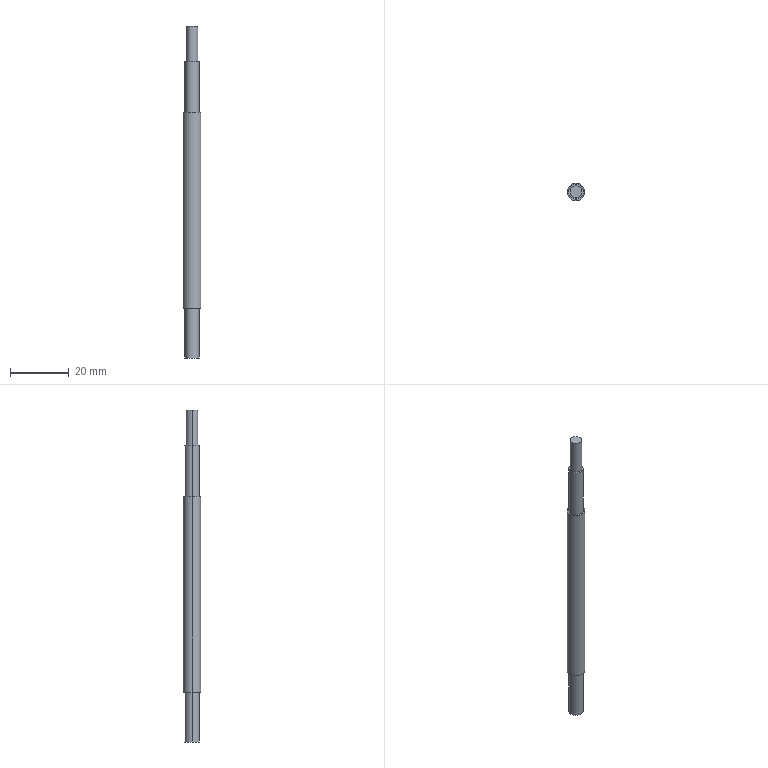Part | SolidWorks | features ICE 3, Extrusion 1 | 1 solid | 13 faces | box 6 x 6 x 113.5 mm | volume 2723 mm3 | cylinder 8 | plane 5 | commonest cylinder face diameters 5 x4 4 x2 6 x2
STEP:
#1=CARTESIAN_POINT('',(2.,0.,113.5));
#2=VERTEX_POINT('',#1);
#3=CARTESIAN_POINT('',(-2.,0.,113.5));
#4=VERTEX_POINT('',#3);
#5=CARTESIAN_POINT('',(0.,0.,113.5));
#6=DIRECTION('',(0.,0.,1.));
#7=DIRECTION('',(1.,0.,0.));
#8=AXIS2_PLACEMENT_3D('',#5,#6,#7);
#9=CIRCLE('',#8,2.);
#10=EDGE_CURVE('',#2,#4,#9,.T.);
#11=ORIENTED_EDGE('',*,*,#10,.F.);
#12=CARTESIAN_POINT('',(2.,0.,101.5));
#13=VERTEX_POINT('',#12);
#14=CARTESIAN_POINT('',(2.,0.,113.5));
#15=DIRECTION('',(0.,0.,-1.));
#16=VECTOR('',#15,1000.);
#17=LINE('',#14,#16);
#18=EDGE_CURVE('',#2,#13,#17,.T.);
#19=ORIENTED_EDGE('',*,*,#18,.T.);
#20=CARTESIAN_POINT('',(-2.,0.,101.5));
#21=VERTEX_POINT('',#20);
#22=CARTESIAN_POINT('',(0.,0.,101.5));
#23=DIRECTION('',(0.,0.,1.));
#24=DIRECTION('',(1.,0.,0.));
#25=AXIS2_PLACEMENT_3D('',#22,#23,#24);
#26=CIRCLE('',#25,2.);
#27=EDGE_CURVE('',#13,#21,#26,.T.);
#28=ORIENTED_EDGE('',*,*,#27,.T.);
#29=CARTESIAN_POINT('',(-2.,0.,113.5));
#30=DIRECTION('',(0.,0.,-1.));
#31=VECTOR('',#30,1000.);
#32=LINE('',#29,#31);
#33=EDGE_CURVE('',#4,#21,#32,.T.);
#34=ORIENTED_EDGE('',*,*,#33,.F.);
#35=EDGE_LOOP('',(#11,#19,#28,#34));
#36=FACE_OUTER_BOUND('',#35,.T.);
#37=CARTESIAN_POINT('',(0.,0.,113.5));
#38=DIRECTION('',(0.,0.,-1.));
#39=DIRECTION('',(-1.,0.,0.));
#40=AXIS2_PLACEMENT_3D('',#37,#38,#39);
#41=CYLINDRICAL_SURFACE('',#40,2.);
#42=ADVANCED_FACE('',(#36),#41,.T.);
#43=CARTESIAN_POINT('',(2.5,0.,101.5));
#44=VERTEX_POINT('',#43);
#45=CARTESIAN_POINT('',(-2.5,0.,101.5));
#46=VERTEX_POINT('',#45);
#47=CARTESIAN_POINT('',(0.,0.,101.5));
#48=DIRECTION('',(0.,0.,1.));
#49=DIRECTION('',(1.,0.,0.));
#50=AXIS2_PLACEMENT_3D('',#47,#48,#49);
#51=CIRCLE('',#50,2.5);
#52=EDGE_CURVE('',#44,#46,#51,.T.);
#53=ORIENTED_EDGE('',*,*,#52,.F.);
#54=CARTESIAN_POINT('',(2.5,0.,84.));
#55=VERTEX_POINT('',#54);
#56=CARTESIAN_POINT('',(2.5,0.,101.5));
#57=DIRECTION('',(0.,0.,-1.));
#58=VECTOR('',#57,1000.);
#59=LINE('',#56,#58);
#60=EDGE_CURVE('',#44,#55,#59,.T.);
#61=ORIENTED_EDGE('',*,*,#60,.T.);
#62=CARTESIAN_POINT('',(-2.5,0.,84.));
#63=VERTEX_POINT('',#62);
#64=CARTESIAN_POINT('',(0.,0.,84.));
#65=DIRECTION('',(0.,0.,1.));
#66=DIRECTION('',(1.,0.,0.));
#67=AXIS2_PLACEMENT_3D('',#64,#65,#66);
#68=CIRCLE('',#67,2.5);
#69=EDGE_CURVE('',#55,#63,#68,.T.);
#70=ORIENTED_EDGE('',*,*,#69,.T.);
#71=CARTESIAN_POINT('',(-2.5,0.,101.5));
#72=DIRECTION('',(0.,0.,-1.));
#73=VECTOR('',#72,1000.);
#74=LINE('',#71,#73);
#75=EDGE_CURVE('',#46,#63,#74,.T.);
#76=ORIENTED_EDGE('',*,*,#75,.F.);
#77=EDGE_LOOP('',(#53,#61,#70,#76));
#78=FACE_OUTER_BOUND('',#77,.T.);
#79=CARTESIAN_POINT('',(0.,0.,101.5));
#80=DIRECTION('',(0.,0.,-1.));
#81=DIRECTION('',(-1.,0.,0.));
#82=AXIS2_PLACEMENT_3D('',#79,#80,#81);
#83=CYLINDRICAL_SURFACE('',#82,2.5);
#84=ADVANCED_FACE('',(#78),#83,.T.);
#85=CARTESIAN_POINT('',(3.,0.,84.));
#86=VERTEX_POINT('',#85);
#87=CARTESIAN_POINT('',(-3.,0.,84.));
#88=VERTEX_POINT('',#87);
#89=CARTESIAN_POINT('',(0.,0.,84.));
#90=DIRECTION('',(0.,0.,1.));
#91=DIRECTION('',(1.,0.,0.));
#92=AXIS2_PLACEMENT_3D('',#89,#90,#91);
#93=CIRCLE('',#92,3.);
#94=EDGE_CURVE('',#86,#88,#93,.T.);
#95=ORIENTED_EDGE('',*,*,#94,.F.);
#96=CARTESIAN_POINT('',(3.,0.,17.));
#97=VERTEX_POINT('',#96);
#98=CARTESIAN_POINT('',(3.,0.,84.));
#99=DIRECTION('',(0.,0.,-1.));
#100=VECTOR('',#99,1000.);
#101=LINE('',#98,#100);
#102=EDGE_CURVE('',#86,#97,#101,.T.);
#103=ORIENTED_EDGE('',*,*,#102,.T.);
#104=CARTESIAN_POINT('',(-3.,0.,17.));
#105=VERTEX_POINT('',#104);
#106=CARTESIAN_POINT('',(0.,0.,17.));
#107=DIRECTION('',(0.,0.,1.));
#108=DIRECTION('',(1.,0.,0.));
#109=AXIS2_PLACEMENT_3D('',#106,#107,#108);
#110=CIRCLE('',#109,3.);
#111=EDGE_CURVE('',#97,#105,#110,.T.);
#112=ORIENTED_EDGE('',*,*,#111,.T.);
#113=CARTESIAN_POINT('',(-3.,0.,84.));
#114=DIRECTION('',(0.,0.,-1.));
#115=VECTOR('',#114,1000.);
#116=LINE('',#113,#115);
#117=EDGE_CURVE('',#88,#105,#116,.T.);
#118=ORIENTED_EDGE('',*,*,#117,.F.);
#119=EDGE_LOOP('',(#95,#103,#112,#118));
#120=FACE_OUTER_BOUND('',#119,.T.);
#121=CARTESIAN_POINT('',(0.,0.,84.));
#122=DIRECTION('',(0.,0.,-1.));
#123=DIRECTION('',(-1.,0.,0.));
#124=AXIS2_PLACEMENT_3D('',#121,#122,#123);
#125=CYLINDRICAL_SURFACE('',#124,3.);
#126=ADVANCED_FACE('',(#120),#125,.T.);
#127=CARTESIAN_POINT('',(2.5,0.,17.));
#128=VERTEX_POINT('',#127);
#129=CARTESIAN_POINT('',(-2.5,0.,17.));
#130=VERTEX_POINT('',#129);
#131=CARTESIAN_POINT('',(0.,0.,17.));
#132=DIRECTION('',(0.,0.,1.));
#133=DIRECTION('',(1.,0.,0.));
#134=AXIS2_PLACEMENT_3D('',#131,#132,#133);
#135=CIRCLE('',#134,2.5);
#136=EDGE_CURVE('',#128,#130,#135,.T.);
#137=ORIENTED_EDGE('',*,*,#136,.F.);
#138=CARTESIAN_POINT('',(2.5,0.,0.));
#139=VERTEX_POINT('',#138);
#140=CARTESIAN_POINT('',(2.5,0.,17.));
#141=DIRECTION('',(0.,0.,-1.));
#142=VECTOR('',#141,1000.);
#143=LINE('',#140,#142);
#144=EDGE_CURVE('',#128,#139,#143,.T.);
#145=ORIENTED_EDGE('',*,*,#144,.T.);
#146=CARTESIAN_POINT('',(-2.5,0.,0.));
#147=VERTEX_POINT('',#146);
#148=CARTESIAN_POINT('',(0.,0.,0.));
#149=DIRECTION('',(0.,0.,1.));
#150=DIRECTION('',(1.,0.,0.));
#151=AXIS2_PLACEMENT_3D('',#148,#149,#150);
#152=CIRCLE('',#151,2.5);
#153=EDGE_CURVE('',#139,#147,#152,.T.);
#154=ORIENTED_EDGE('',*,*,#153,.T.);
#155=CARTESIAN_POINT('',(-2.5,0.,17.));
#156=DIRECTION('',(0.,0.,-1.));
#157=VECTOR('',#156,1000.);
#158=LINE('',#155,#157);
#159=EDGE_CURVE('',#130,#147,#158,.T.);
#160=ORIENTED_EDGE('',*,*,#159,.F.);
#161=EDGE_LOOP('',(#137,#145,#154,#160));
#162=FACE_OUTER_BOUND('',#161,.T.);
#163=CARTESIAN_POINT('',(0.,0.,17.));
#164=DIRECTION('',(0.,0.,-1.));
#165=DIRECTION('',(-1.,0.,0.));
#166=AXIS2_PLACEMENT_3D('',#163,#164,#165);
#167=CYLINDRICAL_SURFACE('',#166,2.5);
#168=ADVANCED_FACE('',(#162),#167,.T.);
#169=ORIENTED_EDGE('',*,*,#144,.F.);
#170=CARTESIAN_POINT('',(0.,0.,17.));
#171=DIRECTION('',(0.,0.,1.));
#172=DIRECTION('',(1.,0.,0.));
#173=AXIS2_PLACEMENT_3D('',#170,#171,#172);
#174=CIRCLE('',#173,2.5);
#175=EDGE_CURVE('',#130,#128,#174,.T.);
#176=ORIENTED_EDGE('',*,*,#175,.F.);
#177=ORIENTED_EDGE('',*,*,#159,.T.);
#178=CARTESIAN_POINT('',(0.,0.,0.));
#179=DIRECTION('',(0.,0.,1.));
#180=DIRECTION('',(1.,0.,0.));
#181=AXIS2_PLACEMENT_3D('',#178,#179,#180);
#182=CIRCLE('',#181,2.5);
#183=EDGE_CURVE('',#147,#139,#182,.T.);
#184=ORIENTED_EDGE('',*,*,#183,.T.);
#185=EDGE_LOOP('',(#169,#176,#177,#184));
#186=FACE_OUTER_BOUND('',#185,.T.);
#187=CARTESIAN_POINT('',(0.,0.,17.));
#188=DIRECTION('',(0.,0.,-1.));
#189=DIRECTION('',(-1.,0.,0.));
#190=AXIS2_PLACEMENT_3D('',#187,#188,#189);
#191=CYLINDRICAL_SURFACE('',#190,2.5);
#192=ADVANCED_FACE('',(#186),#191,.T.);
#193=ORIENTED_EDGE('',*,*,#183,.F.);
#194=ORIENTED_EDGE('',*,*,#153,.F.);
#195=EDGE_LOOP('',(#193,#194));
#196=FACE_OUTER_BOUND('',#195,.T.);
#197=CARTESIAN_POINT('',(0.,0.,0.));
#198=DIRECTION('',(0.,0.,1.));
#199=DIRECTION('',(1.,0.,0.));
#200=AXIS2_PLACEMENT_3D('',#197,#198,#199);
#201=PLANE('',#200);
#202=ADVANCED_FACE('',(#196),#201,.F.);
#203=ORIENTED_EDGE('',*,*,#102,.F.);
#204=CARTESIAN_POINT('',(0.,0.,84.));
#205=DIRECTION('',(0.,0.,1.));
#206=DIRECTION('',(1.,0.,0.));
#207=AXIS2_PLACEMENT_3D('',#204,#205,#206);
#208=CIRCLE('',#207,3.);
#209=EDGE_CURVE('',#88,#86,#208,.T.);
#210=ORIENTED_EDGE('',*,*,#209,.F.);
#211=ORIENTED_EDGE('',*,*,#117,.T.);
#212=CARTESIAN_POINT('',(0.,0.,17.));
#213=DIRECTION('',(0.,0.,1.));
#214=DIRECTION('',(1.,0.,0.));
#215=AXIS2_PLACEMENT_3D('',#212,#213,#214);
#216=CIRCLE('',#215,3.);
#217=EDGE_CURVE('',#105,#97,#216,.T.);
#218=ORIENTED_EDGE('',*,*,#217,.T.);
#219=EDGE_LOOP('',(#203,#210,#211,#218));
#220=FACE_OUTER_BOUND('',#219,.T.);
#221=CARTESIAN_POINT('',(0.,0.,84.));
#222=DIRECTION('',(0.,0.,-1.));
#223=DIRECTION('',(-1.,0.,0.));
#224=AXIS2_PLACEMENT_3D('',#221,#222,#223);
#225=CYLINDRICAL_SURFACE('',#224,3.);
#226=ADVANCED_FACE('',(#220),#225,.T.);
#227=CARTESIAN_POINT('',(0.,0.,84.));
#228=DIRECTION('',(0.,0.,1.));
#229=DIRECTION('',(1.,0.,0.));
#230=AXIS2_PLACEMENT_3D('',#227,#228,#229);
#231=CIRCLE('',#230,2.5);
#232=EDGE_CURVE('',#63,#55,#231,.T.);
#233=ORIENTED_EDGE('',*,*,#232,.F.);
#234=ORIENTED_EDGE('',*,*,#69,.F.);
#235=EDGE_LOOP('',(#233,#234));
#236=FACE_BOUND('',#235,.T.);
#237=ORIENTED_EDGE('',*,*,#209,.T.);
#238=ORIENTED_EDGE('',*,*,#94,.T.);
#239=EDGE_LOOP('',(#237,#238));
#240=FACE_OUTER_BOUND('',#239,.T.);
#241=CARTESIAN_POINT('',(0.,0.,84.));
#242=DIRECTION('',(0.,0.,1.));
#243=DIRECTION('',(1.,0.,0.));
#244=AXIS2_PLACEMENT_3D('',#241,#242,#243);
#245=PLANE('',#244);
#246=ADVANCED_FACE('',(#236,#240),#245,.T.);
#247=ORIENTED_EDGE('',*,*,#175,.T.);
#248=ORIENTED_EDGE('',*,*,#136,.T.);
#249=EDGE_LOOP('',(#247,#248));
#250=FACE_BOUND('',#249,.T.);
#251=ORIENTED_EDGE('',*,*,#217,.F.);
#252=ORIENTED_EDGE('',*,*,#111,.F.);
#253=EDGE_LOOP('',(#251,#252));
#254=FACE_OUTER_BOUND('',#253,.T.);
#255=CARTESIAN_POINT('',(0.,0.,17.));
#256=DIRECTION('',(0.,0.,1.));
#257=DIRECTION('',(1.,0.,0.));
#258=AXIS2_PLACEMENT_3D('',#255,#256,#257);
#259=PLANE('',#258);
#260=ADVANCED_FACE('',(#250,#254),#259,.F.);
#261=ORIENTED_EDGE('',*,*,#60,.F.);
#262=CARTESIAN_POINT('',(0.,0.,101.5));
#263=DIRECTION('',(0.,0.,1.));
#264=DIRECTION('',(1.,0.,0.));
#265=AXIS2_PLACEMENT_3D('',#262,#263,#264);
#266=CIRCLE('',#265,2.5);
#267=EDGE_CURVE('',#46,#44,#266,.T.);
#268=ORIENTED_EDGE('',*,*,#267,.F.);
#269=ORIENTED_EDGE('',*,*,#75,.T.);
#270=ORIENTED_EDGE('',*,*,#232,.T.);
#271=EDGE_LOOP('',(#261,#268,#269,#270));
#272=FACE_OUTER_BOUND('',#271,.T.);
#273=CARTESIAN_POINT('',(0.,0.,101.5));
#274=DIRECTION('',(0.,0.,-1.));
#275=DIRECTION('',(-1.,0.,0.));
#276=AXIS2_PLACEMENT_3D('',#273,#274,#275);
#277=CYLINDRICAL_SURFACE('',#276,2.5);
#278=ADVANCED_FACE('',(#272),#277,.T.);
#279=CARTESIAN_POINT('',(0.,0.,101.5));
#280=DIRECTION('',(0.,0.,1.));
#281=DIRECTION('',(1.,0.,0.));
#282=AXIS2_PLACEMENT_3D('',#279,#280,#281);
#283=CIRCLE('',#282,2.);
#284=EDGE_CURVE('',#21,#13,#283,.T.);
#285=ORIENTED_EDGE('',*,*,#284,.F.);
#286=ORIENTED_EDGE('',*,*,#27,.F.);
#287=EDGE_LOOP('',(#285,#286));
#288=FACE_BOUND('',#287,.T.);
#289=ORIENTED_EDGE('',*,*,#267,.T.);
#290=ORIENTED_EDGE('',*,*,#52,.T.);
#291=EDGE_LOOP('',(#289,#290));
#292=FACE_OUTER_BOUND('',#291,.T.);
#293=CARTESIAN_POINT('',(0.,0.,101.5));
#294=DIRECTION('',(0.,0.,1.));
#295=DIRECTION('',(1.,0.,0.));
#296=AXIS2_PLACEMENT_3D('',#293,#294,#295);
#297=PLANE('',#296);
#298=ADVANCED_FACE('',(#288,#292),#297,.T.);
#299=ORIENTED_EDGE('',*,*,#18,.F.);
#300=CARTESIAN_POINT('',(0.,0.,113.5));
#301=DIRECTION('',(0.,0.,1.));
#302=DIRECTION('',(1.,0.,0.));
#303=AXIS2_PLACEMENT_3D('',#300,#301,#302);
#304=CIRCLE('',#303,2.);
#305=EDGE_CURVE('',#4,#2,#304,.T.);
#306=ORIENTED_EDGE('',*,*,#305,.F.);
#307=ORIENTED_EDGE('',*,*,#33,.T.);
#308=ORIENTED_EDGE('',*,*,#284,.T.);
#309=EDGE_LOOP('',(#299,#306,#307,#308));
#310=FACE_OUTER_BOUND('',#309,.T.);
#311=CARTESIAN_POINT('',(0.,0.,113.5));
#312=DIRECTION('',(0.,0.,-1.));
#313=DIRECTION('',(-1.,0.,0.));
#314=AXIS2_PLACEMENT_3D('',#311,#312,#313);
#315=CYLINDRICAL_SURFACE('',#314,2.);
#316=ADVANCED_FACE('',(#310),#315,.T.);
#317=ORIENTED_EDGE('',*,*,#305,.T.);
#318=ORIENTED_EDGE('',*,*,#10,.T.);
#319=EDGE_LOOP('',(#317,#318));
#320=FACE_OUTER_BOUND('',#319,.T.);
#321=CARTESIAN_POINT('',(0.,0.,113.5));
#322=DIRECTION('',(0.,0.,1.));
#323=DIRECTION('',(1.,0.,0.));
#324=AXIS2_PLACEMENT_3D('',#321,#322,#323);
#325=PLANE('',#324);
#326=ADVANCED_FACE('',(#320),#325,.T.);
#327=CLOSED_SHELL('',(#42,#84,#126,#168,#192,#202,#226,#246,#260,#278,#298,#316,#326));
#328=MANIFOLD_SOLID_BREP('',#327);
#329=CARTESIAN_POINT('',(0.,0.,0.));
#330=DIRECTION('',(0.,0.,1.));
#331=DIRECTION('',(1.,0.,0.));
#332=AXIS2_PLACEMENT_3D('',#329,#330,#331);
#333=(LENGTH_UNIT()NAMED_UNIT(*)SI_UNIT(.MILLI.,.METRE.));
#334=UNCERTAINTY_MEASURE_WITH_UNIT(LENGTH_MEASURE(0.00001),#333,'','');
#335=(NAMED_UNIT(*)PLANE_ANGLE_UNIT()SI_UNIT($,.RADIAN.));
#336=(NAMED_UNIT(*)SI_UNIT($,.STERADIAN.)SOLID_ANGLE_UNIT());
#337=(GEOMETRIC_REPRESENTATION_CONTEXT(3)GLOBAL_UNCERTAINTY_ASSIGNED_CONTEXT((#334))GLOBAL_UNIT_ASSIGNED_CONTEXT((#333,#335,#336))REPRESENTATION_CONTEXT('',''));
#338=ADVANCED_BREP_SHAPE_REPRESENTATION('',(#328,#332),#337);